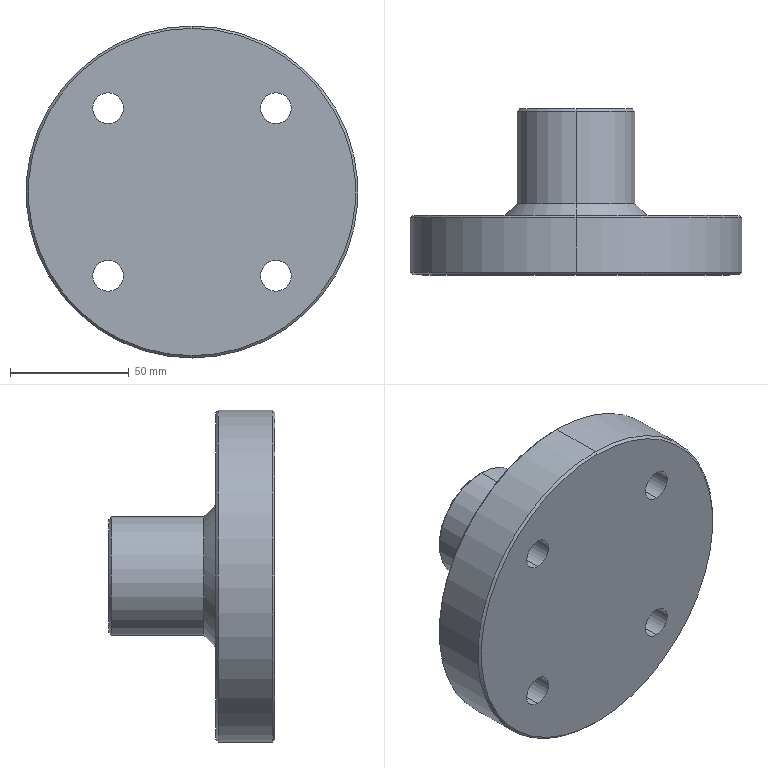Part | SolidWorks | features BaseBody 1 | 1 solid | 30 faces | box 140 x 70 x 140 mm | volume 427164 mm3 | cylinder 14 | cone 12 | plane 4 | commonest cylinder face diameters 13 x8 30 x2 50 x2 140 x2
STEP:
#1=CARTESIAN_POINT('',(35.355,0.,28.855));
#2=VERTEX_POINT('',#1);
#3=CARTESIAN_POINT('',(35.355,0.,41.855));
#4=VERTEX_POINT('',#3);
#5=CARTESIAN_POINT('',(35.355,0.,35.355));
#6=DIRECTION('',(0.,1.,0.));
#7=DIRECTION('',(0.,0.,1.));
#8=AXIS2_PLACEMENT_3D('',#5,#6,#7);
#9=CIRCLE('',#8,6.5);
#10=EDGE_CURVE('',#2,#4,#9,.T.);
#11=ORIENTED_EDGE('',*,*,#10,.F.);
#12=CARTESIAN_POINT('',(35.355,25.,28.855));
#13=VERTEX_POINT('',#12);
#14=CARTESIAN_POINT('',(35.355,25.,28.855));
#15=DIRECTION('',(0.,1.,0.));
#16=VECTOR('',#15,1000.);
#17=LINE('',#14,#16);
#18=EDGE_CURVE('',#2,#13,#17,.T.);
#19=ORIENTED_EDGE('',*,*,#18,.T.);
#20=CARTESIAN_POINT('',(35.355,25.,41.855));
#21=VERTEX_POINT('',#20);
#22=CARTESIAN_POINT('',(35.355,25.,35.355));
#23=DIRECTION('',(0.,1.,0.));
#24=DIRECTION('',(0.,0.,1.));
#25=AXIS2_PLACEMENT_3D('',#22,#23,#24);
#26=CIRCLE('',#25,6.5);
#27=EDGE_CURVE('',#13,#21,#26,.T.);
#28=ORIENTED_EDGE('',*,*,#27,.T.);
#29=CARTESIAN_POINT('',(35.355,25.,41.855));
#30=DIRECTION('',(0.,1.,0.));
#31=VECTOR('',#30,1000.);
#32=LINE('',#29,#31);
#33=EDGE_CURVE('',#4,#21,#32,.T.);
#34=ORIENTED_EDGE('',*,*,#33,.F.);
#35=EDGE_LOOP('',(#11,#19,#28,#34));
#36=FACE_OUTER_BOUND('',#35,.T.);
#37=CARTESIAN_POINT('',(35.355,25.,35.355));
#38=DIRECTION('',(0.,1.,0.));
#39=DIRECTION('',(0.,0.,1.));
#40=AXIS2_PLACEMENT_3D('',#37,#38,#39);
#41=CYLINDRICAL_SURFACE('',#40,6.5);
#42=ADVANCED_FACE('',(#36),#41,.F.);
#43=CARTESIAN_POINT('',(-35.355,0.,28.855));
#44=VERTEX_POINT('',#43);
#45=CARTESIAN_POINT('',(-35.355,0.,41.855));
#46=VERTEX_POINT('',#45);
#47=CARTESIAN_POINT('',(-35.355,0.,35.355));
#48=DIRECTION('',(0.,1.,0.));
#49=DIRECTION('',(0.,0.,1.));
#50=AXIS2_PLACEMENT_3D('',#47,#48,#49);
#51=CIRCLE('',#50,6.5);
#52=EDGE_CURVE('',#44,#46,#51,.T.);
#53=ORIENTED_EDGE('',*,*,#52,.F.);
#54=CARTESIAN_POINT('',(-35.355,25.,28.855));
#55=VERTEX_POINT('',#54);
#56=CARTESIAN_POINT('',(-35.355,25.,28.855));
#57=DIRECTION('',(0.,1.,0.));
#58=VECTOR('',#57,1000.);
#59=LINE('',#56,#58);
#60=EDGE_CURVE('',#44,#55,#59,.T.);
#61=ORIENTED_EDGE('',*,*,#60,.T.);
#62=CARTESIAN_POINT('',(-35.355,25.,41.855));
#63=VERTEX_POINT('',#62);
#64=CARTESIAN_POINT('',(-35.355,25.,35.355));
#65=DIRECTION('',(0.,1.,0.));
#66=DIRECTION('',(0.,0.,1.));
#67=AXIS2_PLACEMENT_3D('',#64,#65,#66);
#68=CIRCLE('',#67,6.5);
#69=EDGE_CURVE('',#55,#63,#68,.T.);
#70=ORIENTED_EDGE('',*,*,#69,.T.);
#71=CARTESIAN_POINT('',(-35.355,25.,41.855));
#72=DIRECTION('',(0.,1.,0.));
#73=VECTOR('',#72,1000.);
#74=LINE('',#71,#73);
#75=EDGE_CURVE('',#46,#63,#74,.T.);
#76=ORIENTED_EDGE('',*,*,#75,.F.);
#77=EDGE_LOOP('',(#53,#61,#70,#76));
#78=FACE_OUTER_BOUND('',#77,.T.);
#79=CARTESIAN_POINT('',(-35.355,25.,35.355));
#80=DIRECTION('',(0.,1.,0.));
#81=DIRECTION('',(0.,0.,1.));
#82=AXIS2_PLACEMENT_3D('',#79,#80,#81);
#83=CYLINDRICAL_SURFACE('',#82,6.5);
#84=ADVANCED_FACE('',(#78),#83,.F.);
#85=CARTESIAN_POINT('',(-35.355,0.,-41.855));
#86=VERTEX_POINT('',#85);
#87=CARTESIAN_POINT('',(-35.355,0.,-28.855));
#88=VERTEX_POINT('',#87);
#89=CARTESIAN_POINT('',(-35.355,0.,-35.355));
#90=DIRECTION('',(0.,1.,0.));
#91=DIRECTION('',(0.,0.,1.));
#92=AXIS2_PLACEMENT_3D('',#89,#90,#91);
#93=CIRCLE('',#92,6.5);
#94=EDGE_CURVE('',#86,#88,#93,.T.);
#95=ORIENTED_EDGE('',*,*,#94,.F.);
#96=CARTESIAN_POINT('',(-35.355,25.,-41.855));
#97=VERTEX_POINT('',#96);
#98=CARTESIAN_POINT('',(-35.355,25.,-41.855));
#99=DIRECTION('',(0.,1.,0.));
#100=VECTOR('',#99,1000.);
#101=LINE('',#98,#100);
#102=EDGE_CURVE('',#86,#97,#101,.T.);
#103=ORIENTED_EDGE('',*,*,#102,.T.);
#104=CARTESIAN_POINT('',(-35.355,25.,-28.855));
#105=VERTEX_POINT('',#104);
#106=CARTESIAN_POINT('',(-35.355,25.,-35.355));
#107=DIRECTION('',(0.,1.,0.));
#108=DIRECTION('',(0.,0.,1.));
#109=AXIS2_PLACEMENT_3D('',#106,#107,#108);
#110=CIRCLE('',#109,6.5);
#111=EDGE_CURVE('',#97,#105,#110,.T.);
#112=ORIENTED_EDGE('',*,*,#111,.T.);
#113=CARTESIAN_POINT('',(-35.355,25.,-28.855));
#114=DIRECTION('',(0.,1.,0.));
#115=VECTOR('',#114,1000.);
#116=LINE('',#113,#115);
#117=EDGE_CURVE('',#88,#105,#116,.T.);
#118=ORIENTED_EDGE('',*,*,#117,.F.);
#119=EDGE_LOOP('',(#95,#103,#112,#118));
#120=FACE_OUTER_BOUND('',#119,.T.);
#121=CARTESIAN_POINT('',(-35.355,25.,-35.355));
#122=DIRECTION('',(0.,1.,0.));
#123=DIRECTION('',(0.,0.,1.));
#124=AXIS2_PLACEMENT_3D('',#121,#122,#123);
#125=CYLINDRICAL_SURFACE('',#124,6.5);
#126=ADVANCED_FACE('',(#120),#125,.F.);
#127=CARTESIAN_POINT('',(35.355,0.,-41.855));
#128=VERTEX_POINT('',#127);
#129=CARTESIAN_POINT('',(35.355,0.,-28.855));
#130=VERTEX_POINT('',#129);
#131=CARTESIAN_POINT('',(35.355,0.,-35.355));
#132=DIRECTION('',(0.,1.,0.));
#133=DIRECTION('',(0.,0.,1.));
#134=AXIS2_PLACEMENT_3D('',#131,#132,#133);
#135=CIRCLE('',#134,6.5);
#136=EDGE_CURVE('',#128,#130,#135,.T.);
#137=ORIENTED_EDGE('',*,*,#136,.F.);
#138=CARTESIAN_POINT('',(35.355,25.,-41.855));
#139=VERTEX_POINT('',#138);
#140=CARTESIAN_POINT('',(35.355,25.,-41.855));
#141=DIRECTION('',(0.,1.,0.));
#142=VECTOR('',#141,1000.);
#143=LINE('',#140,#142);
#144=EDGE_CURVE('',#128,#139,#143,.T.);
#145=ORIENTED_EDGE('',*,*,#144,.T.);
#146=CARTESIAN_POINT('',(35.355,25.,-28.855));
#147=VERTEX_POINT('',#146);
#148=CARTESIAN_POINT('',(35.355,25.,-35.355));
#149=DIRECTION('',(0.,1.,0.));
#150=DIRECTION('',(0.,0.,1.));
#151=AXIS2_PLACEMENT_3D('',#148,#149,#150);
#152=CIRCLE('',#151,6.5);
#153=EDGE_CURVE('',#139,#147,#152,.T.);
#154=ORIENTED_EDGE('',*,*,#153,.T.);
#155=CARTESIAN_POINT('',(35.355,25.,-28.855));
#156=DIRECTION('',(0.,1.,0.));
#157=VECTOR('',#156,1000.);
#158=LINE('',#155,#157);
#159=EDGE_CURVE('',#130,#147,#158,.T.);
#160=ORIENTED_EDGE('',*,*,#159,.F.);
#161=EDGE_LOOP('',(#137,#145,#154,#160));
#162=FACE_OUTER_BOUND('',#161,.T.);
#163=CARTESIAN_POINT('',(35.355,25.,-35.355));
#164=DIRECTION('',(0.,1.,0.));
#165=DIRECTION('',(0.,0.,1.));
#166=AXIS2_PLACEMENT_3D('',#163,#164,#165);
#167=CYLINDRICAL_SURFACE('',#166,6.5);
#168=ADVANCED_FACE('',(#162),#167,.F.);
#169=CARTESIAN_POINT('',(0.,20.,-10.));
#170=VERTEX_POINT('',#169);
#171=CARTESIAN_POINT('',(0.,20.,10.));
#172=VERTEX_POINT('',#171);
#173=CARTESIAN_POINT('',(0.,20.,0.));
#174=DIRECTION('',(0.,1.,0.));
#175=DIRECTION('',(0.,0.,1.));
#176=AXIS2_PLACEMENT_3D('',#173,#174,#175);
#177=CIRCLE('',#176,10.);
#178=EDGE_CURVE('',#170,#172,#177,.T.);
#179=ORIENTED_EDGE('',*,*,#178,.F.);
#180=CARTESIAN_POINT('',(0.,25.,-15.));
#181=VERTEX_POINT('',#180);
#182=CARTESIAN_POINT('',(0.,25.,-15.));
#183=DIRECTION('',(0.,0.7071,-0.7071));
#184=VECTOR('',#183,1000.);
#185=LINE('',#182,#184);
#186=EDGE_CURVE('',#170,#181,#185,.T.);
#187=ORIENTED_EDGE('',*,*,#186,.T.);
#188=CARTESIAN_POINT('',(0.,25.,15.));
#189=VERTEX_POINT('',#188);
#190=CARTESIAN_POINT('',(0.,25.,0.));
#191=DIRECTION('',(0.,1.,0.));
#192=DIRECTION('',(0.,0.,1.));
#193=AXIS2_PLACEMENT_3D('',#190,#191,#192);
#194=CIRCLE('',#193,15.);
#195=EDGE_CURVE('',#181,#189,#194,.T.);
#196=ORIENTED_EDGE('',*,*,#195,.T.);
#197=CARTESIAN_POINT('',(0.,25.,15.));
#198=DIRECTION('',(0.,0.7071,0.7071));
#199=VECTOR('',#198,1000.);
#200=LINE('',#197,#199);
#201=EDGE_CURVE('',#172,#189,#200,.T.);
#202=ORIENTED_EDGE('',*,*,#201,.F.);
#203=EDGE_LOOP('',(#179,#187,#196,#202));
#204=FACE_OUTER_BOUND('',#203,.T.);
#205=CARTESIAN_POINT('',(0.,25.,0.));
#206=DIRECTION('',(0.,1.,0.));
#207=DIRECTION('',(0.,0.,1.));
#208=AXIS2_PLACEMENT_3D('',#205,#206,#207);
#209=CONICAL_SURFACE('',#208,15.,0.7854);
#210=ADVANCED_FACE('',(#204),#209,.F.);
#211=ORIENTED_EDGE('',*,*,#195,.F.);
#212=CARTESIAN_POINT('',(0.,69.,-15.));
#213=VERTEX_POINT('',#212);
#214=CARTESIAN_POINT('',(0.,20.,-15.));
#215=DIRECTION('',(0.,1.,0.));
#216=VECTOR('',#215,1000.);
#217=LINE('',#214,#216);
#218=EDGE_CURVE('',#181,#213,#217,.T.);
#219=ORIENTED_EDGE('',*,*,#218,.T.);
#220=CARTESIAN_POINT('',(0.,69.,15.));
#221=VERTEX_POINT('',#220);
#222=CARTESIAN_POINT('',(0.,69.,0.));
#223=DIRECTION('',(0.,1.,0.));
#224=DIRECTION('',(0.,0.,1.));
#225=AXIS2_PLACEMENT_3D('',#222,#223,#224);
#226=CIRCLE('',#225,15.);
#227=EDGE_CURVE('',#213,#221,#226,.T.);
#228=ORIENTED_EDGE('',*,*,#227,.T.);
#229=CARTESIAN_POINT('',(0.,20.,15.));
#230=DIRECTION('',(0.,1.,0.));
#231=VECTOR('',#230,1000.);
#232=LINE('',#229,#231);
#233=EDGE_CURVE('',#189,#221,#232,.T.);
#234=ORIENTED_EDGE('',*,*,#233,.F.);
#235=EDGE_LOOP('',(#211,#219,#228,#234));
#236=FACE_OUTER_BOUND('',#235,.T.);
#237=CARTESIAN_POINT('',(0.,20.,0.));
#238=DIRECTION('',(0.,1.,0.));
#239=DIRECTION('',(0.,0.,1.));
#240=AXIS2_PLACEMENT_3D('',#237,#238,#239);
#241=CYLINDRICAL_SURFACE('',#240,15.);
#242=ADVANCED_FACE('',(#236),#241,.F.);
#243=ORIENTED_EDGE('',*,*,#227,.F.);
#244=CARTESIAN_POINT('',(0.,70.,-16.));
#245=VERTEX_POINT('',#244);
#246=CARTESIAN_POINT('',(0.,70.,-16.));
#247=DIRECTION('',(0.,0.7071,-0.7071));
#248=VECTOR('',#247,1000.);
#249=LINE('',#246,#248);
#250=EDGE_CURVE('',#213,#245,#249,.T.);
#251=ORIENTED_EDGE('',*,*,#250,.T.);
#252=CARTESIAN_POINT('',(0.,70.,16.));
#253=VERTEX_POINT('',#252);
#254=CARTESIAN_POINT('',(0.,70.,0.));
#255=DIRECTION('',(0.,1.,0.));
#256=DIRECTION('',(0.,0.,1.));
#257=AXIS2_PLACEMENT_3D('',#254,#255,#256);
#258=CIRCLE('',#257,16.);
#259=EDGE_CURVE('',#245,#253,#258,.T.);
#260=ORIENTED_EDGE('',*,*,#259,.T.);
#261=CARTESIAN_POINT('',(0.,70.,16.));
#262=DIRECTION('',(0.,0.7071,0.7071));
#263=VECTOR('',#262,1000.);
#264=LINE('',#261,#263);
#265=EDGE_CURVE('',#221,#253,#264,.T.);
#266=ORIENTED_EDGE('',*,*,#265,.F.);
#267=EDGE_LOOP('',(#243,#251,#260,#266));
#268=FACE_OUTER_BOUND('',#267,.T.);
#269=CARTESIAN_POINT('',(0.,70.,0.));
#270=DIRECTION('',(0.,1.,0.));
#271=DIRECTION('',(0.,0.,1.));
#272=AXIS2_PLACEMENT_3D('',#269,#270,#271);
#273=CONICAL_SURFACE('',#272,16.,0.7854);
#274=ADVANCED_FACE('',(#268),#273,.F.);
#275=CARTESIAN_POINT('',(0.,70.,24.));
#276=VERTEX_POINT('',#275);
#277=CARTESIAN_POINT('',(0.,70.,-24.));
#278=VERTEX_POINT('',#277);
#279=CARTESIAN_POINT('',(0.,70.,0.));
#280=DIRECTION('',(0.,1.,0.));
#281=DIRECTION('',(0.,0.,1.));
#282=AXIS2_PLACEMENT_3D('',#279,#280,#281);
#283=CIRCLE('',#282,24.);
#284=EDGE_CURVE('',#276,#278,#283,.T.);
#285=ORIENTED_EDGE('',*,*,#284,.F.);
#286=CARTESIAN_POINT('',(0.,69.,25.));
#287=VERTEX_POINT('',#286);
#288=CARTESIAN_POINT('',(0.,69.,25.));
#289=DIRECTION('',(0.,-0.7071,0.7071));
#290=VECTOR('',#289,1000.);
#291=LINE('',#288,#290);
#292=EDGE_CURVE('',#276,#287,#291,.T.);
#293=ORIENTED_EDGE('',*,*,#292,.T.);
#294=CARTESIAN_POINT('',(0.,69.,-25.));
#295=VERTEX_POINT('',#294);
#296=CARTESIAN_POINT('',(0.,69.,0.));
#297=DIRECTION('',(0.,1.,0.));
#298=DIRECTION('',(0.,0.,1.));
#299=AXIS2_PLACEMENT_3D('',#296,#297,#298);
#300=CIRCLE('',#299,25.);
#301=EDGE_CURVE('',#287,#295,#300,.T.);
#302=ORIENTED_EDGE('',*,*,#301,.T.);
#303=CARTESIAN_POINT('',(0.,69.,-25.));
#304=DIRECTION('',(0.,-0.7071,-0.7071));
#305=VECTOR('',#304,1000.);
#306=LINE('',#303,#305);
#307=EDGE_CURVE('',#278,#295,#306,.T.);
#308=ORIENTED_EDGE('',*,*,#307,.F.);
#309=EDGE_LOOP('',(#285,#293,#302,#308));
#310=FACE_OUTER_BOUND('',#309,.T.);
#311=CARTESIAN_POINT('',(0.,69.,0.));
#312=DIRECTION('',(0.,-1.,0.));
#313=DIRECTION('',(0.,0.,-1.));
#314=AXIS2_PLACEMENT_3D('',#311,#312,#313);
#315=CONICAL_SURFACE('',#314,25.,0.7854);
#316=ADVANCED_FACE('',(#310),#315,.T.);
#317=CARTESIAN_POINT('',(0.,30.,25.));
#318=VERTEX_POINT('',#317);
#319=CARTESIAN_POINT('',(0.,30.,-25.));
#320=VERTEX_POINT('',#319);
#321=CARTESIAN_POINT('',(0.,30.,0.));
#322=DIRECTION('',(0.,1.,0.));
#323=DIRECTION('',(0.,0.,1.));
#324=AXIS2_PLACEMENT_3D('',#321,#322,#323);
#325=CIRCLE('',#324,25.);
#326=EDGE_CURVE('',#318,#320,#325,.T.);
#327=ORIENTED_EDGE('',*,*,#326,.T.);
#328=CARTESIAN_POINT('',(0.,20.,-25.));
#329=DIRECTION('',(0.,1.,0.));
#330=VECTOR('',#329,1000.);
#331=LINE('',#328,#330);
#332=EDGE_CURVE('',#320,#295,#331,.T.);
#333=ORIENTED_EDGE('',*,*,#332,.T.);
#334=ORIENTED_EDGE('',*,*,#301,.F.);
#335=CARTESIAN_POINT('',(0.,20.,25.));
#336=DIRECTION('',(0.,1.,0.));
#337=VECTOR('',#336,1000.);
#338=LINE('',#335,#337);
#339=EDGE_CURVE('',#318,#287,#338,.T.);
#340=ORIENTED_EDGE('',*,*,#339,.F.);
#341=EDGE_LOOP('',(#327,#333,#334,#340));
#342=FACE_OUTER_BOUND('',#341,.T.);
#343=CARTESIAN_POINT('',(0.,20.,0.));
#344=DIRECTION('',(0.,1.,0.));
#345=DIRECTION('',(0.,0.,1.));
#346=AXIS2_PLACEMENT_3D('',#343,#344,#345);
#347=CYLINDRICAL_SURFACE('',#346,25.);
#348=ADVANCED_FACE('',(#342),#347,.T.);
#349=ORIENTED_EDGE('',*,*,#326,.F.);
#350=CARTESIAN_POINT('',(0.,25.,30.));
#351=VERTEX_POINT('',#350);
#352=CARTESIAN_POINT('',(0.,25.,30.));
#353=DIRECTION('',(0.,-0.7071,0.7071));
#354=VECTOR('',#353,1000.);
#355=LINE('',#352,#354);
#356=EDGE_CURVE('',#318,#351,#355,.T.);
#357=ORIENTED_EDGE('',*,*,#356,.T.);
#358=CARTESIAN_POINT('',(0.,25.,-30.));
#359=VERTEX_POINT('',#358);
#360=CARTESIAN_POINT('',(0.,25.,0.));
#361=DIRECTION('',(0.,1.,0.));
#362=DIRECTION('',(0.,0.,1.));
#363=AXIS2_PLACEMENT_3D('',#360,#361,#362);
#364=CIRCLE('',#363,30.);
#365=EDGE_CURVE('',#351,#359,#364,.T.);
#366=ORIENTED_EDGE('',*,*,#365,.T.);
#367=CARTESIAN_POINT('',(0.,25.,-30.));
#368=DIRECTION('',(0.,-0.7071,-0.7071));
#369=VECTOR('',#368,1000.);
#370=LINE('',#367,#369);
#371=EDGE_CURVE('',#320,#359,#370,.T.);
#372=ORIENTED_EDGE('',*,*,#371,.F.);
#373=EDGE_LOOP('',(#349,#357,#366,#372));
#374=FACE_OUTER_BOUND('',#373,.T.);
#375=CARTESIAN_POINT('',(0.,25.,0.));
#376=DIRECTION('',(0.,-1.,0.));
#377=DIRECTION('',(0.,0.,-1.));
#378=AXIS2_PLACEMENT_3D('',#375,#376,#377);
#379=CONICAL_SURFACE('',#378,30.,0.7854);
#380=ADVANCED_FACE('',(#374),#379,.T.);
#381=CARTESIAN_POINT('',(0.,25.,69.));
#382=VERTEX_POINT('',#381);
#383=CARTESIAN_POINT('',(0.,25.,-69.));
#384=VERTEX_POINT('',#383);
#385=CARTESIAN_POINT('',(0.,25.,0.));
#386=DIRECTION('',(0.,1.,0.));
#387=DIRECTION('',(0.,0.,1.));
#388=AXIS2_PLACEMENT_3D('',#385,#386,#387);
#389=CIRCLE('',#388,69.);
#390=EDGE_CURVE('',#382,#384,#389,.T.);
#391=ORIENTED_EDGE('',*,*,#390,.F.);
#392=CARTESIAN_POINT('',(0.,24.,70.));
#393=VERTEX_POINT('',#392);
#394=CARTESIAN_POINT('',(0.,24.,70.));
#395=DIRECTION('',(0.,-0.7071,0.7071));
#396=VECTOR('',#395,1000.);
#397=LINE('',#394,#396);
#398=EDGE_CURVE('',#382,#393,#397,.T.);
#399=ORIENTED_EDGE('',*,*,#398,.T.);
#400=CARTESIAN_POINT('',(0.,24.,-70.));
#401=VERTEX_POINT('',#400);
#402=CARTESIAN_POINT('',(0.,24.,0.));
#403=DIRECTION('',(0.,1.,0.));
#404=DIRECTION('',(0.,0.,1.));
#405=AXIS2_PLACEMENT_3D('',#402,#403,#404);
#406=CIRCLE('',#405,70.);
#407=EDGE_CURVE('',#393,#401,#406,.T.);
#408=ORIENTED_EDGE('',*,*,#407,.T.);
#409=CARTESIAN_POINT('',(0.,24.,-70.));
#410=DIRECTION('',(0.,-0.7071,-0.7071));
#411=VECTOR('',#410,1000.);
#412=LINE('',#409,#411);
#413=EDGE_CURVE('',#384,#401,#412,.T.);
#414=ORIENTED_EDGE('',*,*,#413,.F.);
#415=EDGE_LOOP('',(#391,#399,#408,#414));
#416=FACE_OUTER_BOUND('',#415,.T.);
#417=CARTESIAN_POINT('',(0.,24.,0.));
#418=DIRECTION('',(0.,-1.,0.));
#419=DIRECTION('',(0.,0.,-1.));
#420=AXIS2_PLACEMENT_3D('',#417,#418,#419);
#421=CONICAL_SURFACE('',#420,70.,0.7854);
#422=ADVANCED_FACE('',(#416),#421,.T.);
#423=CARTESIAN_POINT('',(0.,1.,70.));
#424=VERTEX_POINT('',#423);
#425=CARTESIAN_POINT('',(0.,1.,-70.));
#426=VERTEX_POINT('',#425);
#427=CARTESIAN_POINT('',(0.,1.,0.));
#428=DIRECTION('',(0.,1.,0.));
#429=DIRECTION('',(0.,0.,1.));
#430=AXIS2_PLACEMENT_3D('',#427,#428,#429);
#431=CIRCLE('',#430,70.);
#432=EDGE_CURVE('',#424,#426,#431,.T.);
#433=ORIENTED_EDGE('',*,*,#432,.T.);
#434=CARTESIAN_POINT('',(0.,20.,-70.));
#435=DIRECTION('',(0.,1.,0.));
#436=VECTOR('',#435,1000.);
#437=LINE('',#434,#436);
#438=EDGE_CURVE('',#426,#401,#437,.T.);
#439=ORIENTED_EDGE('',*,*,#438,.T.);
#440=ORIENTED_EDGE('',*,*,#407,.F.);
#441=CARTESIAN_POINT('',(0.,20.,70.));
#442=DIRECTION('',(0.,1.,0.));
#443=VECTOR('',#442,1000.);
#444=LINE('',#441,#443);
#445=EDGE_CURVE('',#424,#393,#444,.T.);
#446=ORIENTED_EDGE('',*,*,#445,.F.);
#447=EDGE_LOOP('',(#433,#439,#440,#446));
#448=FACE_OUTER_BOUND('',#447,.T.);
#449=CARTESIAN_POINT('',(0.,20.,0.));
#450=DIRECTION('',(0.,1.,0.));
#451=DIRECTION('',(0.,0.,1.));
#452=AXIS2_PLACEMENT_3D('',#449,#450,#451);
#453=CYLINDRICAL_SURFACE('',#452,70.);
#454=ADVANCED_FACE('',(#448),#453,.T.);
#455=CARTESIAN_POINT('',(0.,0.,69.));
#456=VERTEX_POINT('',#455);
#457=CARTESIAN_POINT('',(0.,0.,-69.));
#458=VERTEX_POINT('',#457);
#459=CARTESIAN_POINT('',(0.,0.,0.));
#460=DIRECTION('',(0.,1.,0.));
#461=DIRECTION('',(0.,0.,1.));
#462=AXIS2_PLACEMENT_3D('',#459,#460,#461);
#463=CIRCLE('',#462,69.);
#464=EDGE_CURVE('',#456,#458,#463,.T.);
#465=ORIENTED_EDGE('',*,*,#464,.T.);
#466=CARTESIAN_POINT('',(0.,0.,-69.));
#467=DIRECTION('',(0.,0.7071,-0.7071));
#468=VECTOR('',#467,1000.);
#469=LINE('',#466,#468);
#470=EDGE_CURVE('',#458,#426,#469,.T.);
#471=ORIENTED_EDGE('',*,*,#470,.T.);
#472=ORIENTED_EDGE('',*,*,#432,.F.);
#473=CARTESIAN_POINT('',(0.,0.,69.));
#474=DIRECTION('',(0.,0.7071,0.7071));
#475=VECTOR('',#474,1000.);
#476=LINE('',#473,#475);
#477=EDGE_CURVE('',#456,#424,#476,.T.);
#478=ORIENTED_EDGE('',*,*,#477,.F.);
#479=EDGE_LOOP('',(#465,#471,#472,#478));
#480=FACE_OUTER_BOUND('',#479,.T.);
#481=CARTESIAN_POINT('',(0.,0.,0.));
#482=DIRECTION('',(0.,1.,0.));
#483=DIRECTION('',(0.,0.,1.));
#484=AXIS2_PLACEMENT_3D('',#481,#482,#483);
#485=CONICAL_SURFACE('',#484,69.,0.7854);
#486=ADVANCED_FACE('',(#480),#485,.T.);
#487=CARTESIAN_POINT('',(35.355,0.,35.355));
#488=DIRECTION('',(0.,1.,0.));
#489=DIRECTION('',(0.,0.,1.));
#490=AXIS2_PLACEMENT_3D('',#487,#488,#489);
#491=CIRCLE('',#490,6.5);
#492=EDGE_CURVE('',#4,#2,#491,.T.);
#493=ORIENTED_EDGE('',*,*,#492,.T.);
#494=ORIENTED_EDGE('',*,*,#10,.T.);
#495=EDGE_LOOP('',(#493,#494));
#496=FACE_BOUND('',#495,.T.);
#497=CARTESIAN_POINT('',(-35.355,0.,35.355));
#498=DIRECTION('',(0.,1.,0.));
#499=DIRECTION('',(0.,0.,1.));
#500=AXIS2_PLACEMENT_3D('',#497,#498,#499);
#501=CIRCLE('',#500,6.5);
#502=EDGE_CURVE('',#46,#44,#501,.T.);
#503=ORIENTED_EDGE('',*,*,#502,.T.);
#504=ORIENTED_EDGE('',*,*,#52,.T.);
#505=EDGE_LOOP('',(#503,#504));
#506=FACE_BOUND('',#505,.T.);
#507=CARTESIAN_POINT('',(-35.355,0.,-35.355));
#508=DIRECTION('',(0.,1.,0.));
#509=DIRECTION('',(0.,0.,1.));
#510=AXIS2_PLACEMENT_3D('',#507,#508,#509);
#511=CIRCLE('',#510,6.5);
#512=EDGE_CURVE('',#88,#86,#511,.T.);
#513=ORIENTED_EDGE('',*,*,#512,.T.);
#514=ORIENTED_EDGE('',*,*,#94,.T.);
#515=EDGE_LOOP('',(#513,#514));
#516=FACE_BOUND('',#515,.T.);
#517=CARTESIAN_POINT('',(35.355,0.,-35.355));
#518=DIRECTION('',(0.,1.,0.));
#519=DIRECTION('',(0.,0.,1.));
#520=AXIS2_PLACEMENT_3D('',#517,#518,#519);
#521=CIRCLE('',#520,6.5);
#522=EDGE_CURVE('',#130,#128,#521,.T.);
#523=ORIENTED_EDGE('',*,*,#522,.T.);
#524=ORIENTED_EDGE('',*,*,#136,.T.);
#525=EDGE_LOOP('',(#523,#524));
#526=FACE_BOUND('',#525,.T.);
#527=ORIENTED_EDGE('',*,*,#464,.F.);
#528=CARTESIAN_POINT('',(0.,0.,0.));
#529=DIRECTION('',(0.,1.,0.));
#530=DIRECTION('',(0.,0.,1.));
#531=AXIS2_PLACEMENT_3D('',#528,#529,#530);
#532=CIRCLE('',#531,69.);
#533=EDGE_CURVE('',#458,#456,#532,.T.);
#534=ORIENTED_EDGE('',*,*,#533,.F.);
#535=EDGE_LOOP('',(#527,#534));
#536=FACE_OUTER_BOUND('',#535,.T.);
#537=CARTESIAN_POINT('',(0.,0.,0.));
#538=DIRECTION('',(0.,1.,0.));
#539=DIRECTION('',(0.,0.,1.));
#540=AXIS2_PLACEMENT_3D('',#537,#538,#539);
#541=PLANE('',#540);
#542=ADVANCED_FACE('',(#496,#506,#516,#526,#536),#541,.F.);
#543=ORIENTED_EDGE('',*,*,#470,.F.);
#544=ORIENTED_EDGE('',*,*,#533,.T.);
#545=ORIENTED_EDGE('',*,*,#477,.T.);
#546=CARTESIAN_POINT('',(0.,1.,0.));
#547=DIRECTION('',(0.,1.,0.));
#548=DIRECTION('',(0.,0.,1.));
#549=AXIS2_PLACEMENT_3D('',#546,#547,#548);
#550=CIRCLE('',#549,70.);
#551=EDGE_CURVE('',#426,#424,#550,.T.);
#552=ORIENTED_EDGE('',*,*,#551,.F.);
#553=EDGE_LOOP('',(#543,#544,#545,#552));
#554=FACE_OUTER_BOUND('',#553,.T.);
#555=CARTESIAN_POINT('',(0.,0.,0.));
#556=DIRECTION('',(0.,1.,0.));
#557=DIRECTION('',(0.,0.,1.));
#558=AXIS2_PLACEMENT_3D('',#555,#556,#557);
#559=CONICAL_SURFACE('',#558,69.,0.7854);
#560=ADVANCED_FACE('',(#554),#559,.T.);
#561=ORIENTED_EDGE('',*,*,#438,.F.);
#562=ORIENTED_EDGE('',*,*,#551,.T.);
#563=ORIENTED_EDGE('',*,*,#445,.T.);
#564=CARTESIAN_POINT('',(0.,24.,0.));
#565=DIRECTION('',(0.,1.,0.));
#566=DIRECTION('',(0.,0.,1.));
#567=AXIS2_PLACEMENT_3D('',#564,#565,#566);
#568=CIRCLE('',#567,70.);
#569=EDGE_CURVE('',#401,#393,#568,.T.);
#570=ORIENTED_EDGE('',*,*,#569,.F.);
#571=EDGE_LOOP('',(#561,#562,#563,#570));
#572=FACE_OUTER_BOUND('',#571,.T.);
#573=CARTESIAN_POINT('',(0.,20.,0.));
#574=DIRECTION('',(0.,1.,0.));
#575=DIRECTION('',(0.,0.,1.));
#576=AXIS2_PLACEMENT_3D('',#573,#574,#575);
#577=CYLINDRICAL_SURFACE('',#576,70.);
#578=ADVANCED_FACE('',(#572),#577,.T.);
#579=ORIENTED_EDGE('',*,*,#398,.F.);
#580=CARTESIAN_POINT('',(0.,25.,0.));
#581=DIRECTION('',(0.,1.,0.));
#582=DIRECTION('',(0.,0.,1.));
#583=AXIS2_PLACEMENT_3D('',#580,#581,#582);
#584=CIRCLE('',#583,69.);
#585=EDGE_CURVE('',#384,#382,#584,.T.);
#586=ORIENTED_EDGE('',*,*,#585,.F.);
#587=ORIENTED_EDGE('',*,*,#413,.T.);
#588=ORIENTED_EDGE('',*,*,#569,.T.);
#589=EDGE_LOOP('',(#579,#586,#587,#588));
#590=FACE_OUTER_BOUND('',#589,.T.);
#591=CARTESIAN_POINT('',(0.,24.,0.));
#592=DIRECTION('',(0.,-1.,0.));
#593=DIRECTION('',(0.,0.,-1.));
#594=AXIS2_PLACEMENT_3D('',#591,#592,#593);
#595=CONICAL_SURFACE('',#594,70.,0.7854);
#596=ADVANCED_FACE('',(#590),#595,.T.);
#597=CARTESIAN_POINT('',(35.355,25.,35.355));
#598=DIRECTION('',(0.,1.,0.));
#599=DIRECTION('',(0.,0.,1.));
#600=AXIS2_PLACEMENT_3D('',#597,#598,#599);
#601=CIRCLE('',#600,6.5);
#602=EDGE_CURVE('',#21,#13,#601,.T.);
#603=ORIENTED_EDGE('',*,*,#602,.F.);
#604=ORIENTED_EDGE('',*,*,#27,.F.);
#605=EDGE_LOOP('',(#603,#604));
#606=FACE_BOUND('',#605,.T.);
#607=CARTESIAN_POINT('',(-35.355,25.,35.355));
#608=DIRECTION('',(0.,1.,0.));
#609=DIRECTION('',(0.,0.,1.));
#610=AXIS2_PLACEMENT_3D('',#607,#608,#609);
#611=CIRCLE('',#610,6.5);
#612=EDGE_CURVE('',#63,#55,#611,.T.);
#613=ORIENTED_EDGE('',*,*,#612,.F.);
#614=ORIENTED_EDGE('',*,*,#69,.F.);
#615=EDGE_LOOP('',(#613,#614));
#616=FACE_BOUND('',#615,.T.);
#617=CARTESIAN_POINT('',(-35.355,25.,-35.355));
#618=DIRECTION('',(0.,1.,0.));
#619=DIRECTION('',(0.,0.,1.));
#620=AXIS2_PLACEMENT_3D('',#617,#618,#619);
#621=CIRCLE('',#620,6.5);
#622=EDGE_CURVE('',#105,#97,#621,.T.);
#623=ORIENTED_EDGE('',*,*,#622,.F.);
#624=ORIENTED_EDGE('',*,*,#111,.F.);
#625=EDGE_LOOP('',(#623,#624));
#626=FACE_BOUND('',#625,.T.);
#627=CARTESIAN_POINT('',(35.355,25.,-35.355));
#628=DIRECTION('',(0.,1.,0.));
#629=DIRECTION('',(0.,0.,1.));
#630=AXIS2_PLACEMENT_3D('',#627,#628,#629);
#631=CIRCLE('',#630,6.5);
#632=EDGE_CURVE('',#147,#139,#631,.T.);
#633=ORIENTED_EDGE('',*,*,#632,.F.);
#634=ORIENTED_EDGE('',*,*,#153,.F.);
#635=EDGE_LOOP('',(#633,#634));
#636=FACE_BOUND('',#635,.T.);
#637=CARTESIAN_POINT('',(0.,25.,0.));
#638=DIRECTION('',(0.,1.,0.));
#639=DIRECTION('',(0.,0.,1.));
#640=AXIS2_PLACEMENT_3D('',#637,#638,#639);
#641=CIRCLE('',#640,30.);
#642=EDGE_CURVE('',#359,#351,#641,.T.);
#643=ORIENTED_EDGE('',*,*,#642,.F.);
#644=ORIENTED_EDGE('',*,*,#365,.F.);
#645=EDGE_LOOP('',(#643,#644));
#646=FACE_BOUND('',#645,.T.);
#647=ORIENTED_EDGE('',*,*,#585,.T.);
#648=ORIENTED_EDGE('',*,*,#390,.T.);
#649=EDGE_LOOP('',(#647,#648));
#650=FACE_OUTER_BOUND('',#649,.T.);
#651=CARTESIAN_POINT('',(69.,25.,0.));
#652=DIRECTION('',(0.,-1.,0.));
#653=DIRECTION('',(0.,0.,-1.));
#654=AXIS2_PLACEMENT_3D('',#651,#652,#653);
#655=PLANE('',#654);
#656=ADVANCED_FACE('',(#606,#616,#626,#636,#646,#650),#655,.F.);
#657=ORIENTED_EDGE('',*,*,#356,.F.);
#658=CARTESIAN_POINT('',(0.,30.,0.));
#659=DIRECTION('',(0.,1.,0.));
#660=DIRECTION('',(0.,0.,1.));
#661=AXIS2_PLACEMENT_3D('',#658,#659,#660);
#662=CIRCLE('',#661,25.);
#663=EDGE_CURVE('',#320,#318,#662,.T.);
#664=ORIENTED_EDGE('',*,*,#663,.F.);
#665=ORIENTED_EDGE('',*,*,#371,.T.);
#666=ORIENTED_EDGE('',*,*,#642,.T.);
#667=EDGE_LOOP('',(#657,#664,#665,#666));
#668=FACE_OUTER_BOUND('',#667,.T.);
#669=CARTESIAN_POINT('',(0.,25.,0.));
#670=DIRECTION('',(0.,-1.,0.));
#671=DIRECTION('',(0.,0.,-1.));
#672=AXIS2_PLACEMENT_3D('',#669,#670,#671);
#673=CONICAL_SURFACE('',#672,30.,0.7854);
#674=ADVANCED_FACE('',(#668),#673,.T.);
#675=ORIENTED_EDGE('',*,*,#332,.F.);
#676=ORIENTED_EDGE('',*,*,#663,.T.);
#677=ORIENTED_EDGE('',*,*,#339,.T.);
#678=CARTESIAN_POINT('',(0.,69.,0.));
#679=DIRECTION('',(0.,1.,0.));
#680=DIRECTION('',(0.,0.,1.));
#681=AXIS2_PLACEMENT_3D('',#678,#679,#680);
#682=CIRCLE('',#681,25.);
#683=EDGE_CURVE('',#295,#287,#682,.T.);
#684=ORIENTED_EDGE('',*,*,#683,.F.);
#685=EDGE_LOOP('',(#675,#676,#677,#684));
#686=FACE_OUTER_BOUND('',#685,.T.);
#687=CARTESIAN_POINT('',(0.,20.,0.));
#688=DIRECTION('',(0.,1.,0.));
#689=DIRECTION('',(0.,0.,1.));
#690=AXIS2_PLACEMENT_3D('',#687,#688,#689);
#691=CYLINDRICAL_SURFACE('',#690,25.);
#692=ADVANCED_FACE('',(#686),#691,.T.);
#693=ORIENTED_EDGE('',*,*,#292,.F.);
#694=CARTESIAN_POINT('',(0.,70.,0.));
#695=DIRECTION('',(0.,1.,0.));
#696=DIRECTION('',(0.,0.,1.));
#697=AXIS2_PLACEMENT_3D('',#694,#695,#696);
#698=CIRCLE('',#697,24.);
#699=EDGE_CURVE('',#278,#276,#698,.T.);
#700=ORIENTED_EDGE('',*,*,#699,.F.);
#701=ORIENTED_EDGE('',*,*,#307,.T.);
#702=ORIENTED_EDGE('',*,*,#683,.T.);
#703=EDGE_LOOP('',(#693,#700,#701,#702));
#704=FACE_OUTER_BOUND('',#703,.T.);
#705=CARTESIAN_POINT('',(0.,69.,0.));
#706=DIRECTION('',(0.,-1.,0.));
#707=DIRECTION('',(0.,0.,-1.));
#708=AXIS2_PLACEMENT_3D('',#705,#706,#707);
#709=CONICAL_SURFACE('',#708,25.,0.7854);
#710=ADVANCED_FACE('',(#704),#709,.T.);
#711=CARTESIAN_POINT('',(0.,70.,0.));
#712=DIRECTION('',(0.,1.,0.));
#713=DIRECTION('',(0.,0.,1.));
#714=AXIS2_PLACEMENT_3D('',#711,#712,#713);
#715=CIRCLE('',#714,16.);
#716=EDGE_CURVE('',#253,#245,#715,.T.);
#717=ORIENTED_EDGE('',*,*,#716,.F.);
#718=ORIENTED_EDGE('',*,*,#259,.F.);
#719=EDGE_LOOP('',(#717,#718));
#720=FACE_BOUND('',#719,.T.);
#721=ORIENTED_EDGE('',*,*,#699,.T.);
#722=ORIENTED_EDGE('',*,*,#284,.T.);
#723=EDGE_LOOP('',(#721,#722));
#724=FACE_OUTER_BOUND('',#723,.T.);
#725=CARTESIAN_POINT('',(24.,70.,0.));
#726=DIRECTION('',(0.,-1.,0.));
#727=DIRECTION('',(0.,0.,-1.));
#728=AXIS2_PLACEMENT_3D('',#725,#726,#727);
#729=PLANE('',#728);
#730=ADVANCED_FACE('',(#720,#724),#729,.F.);
#731=ORIENTED_EDGE('',*,*,#250,.F.);
#732=CARTESIAN_POINT('',(0.,69.,0.));
#733=DIRECTION('',(0.,1.,0.));
#734=DIRECTION('',(0.,0.,1.));
#735=AXIS2_PLACEMENT_3D('',#732,#733,#734);
#736=CIRCLE('',#735,15.);
#737=EDGE_CURVE('',#221,#213,#736,.T.);
#738=ORIENTED_EDGE('',*,*,#737,.F.);
#739=ORIENTED_EDGE('',*,*,#265,.T.);
#740=ORIENTED_EDGE('',*,*,#716,.T.);
#741=EDGE_LOOP('',(#731,#738,#739,#740));
#742=FACE_OUTER_BOUND('',#741,.T.);
#743=CARTESIAN_POINT('',(0.,70.,0.));
#744=DIRECTION('',(0.,1.,0.));
#745=DIRECTION('',(0.,0.,1.));
#746=AXIS2_PLACEMENT_3D('',#743,#744,#745);
#747=CONICAL_SURFACE('',#746,16.,0.7854);
#748=ADVANCED_FACE('',(#742),#747,.F.);
#749=ORIENTED_EDGE('',*,*,#218,.F.);
#750=CARTESIAN_POINT('',(0.,25.,0.));
#751=DIRECTION('',(0.,1.,0.));
#752=DIRECTION('',(0.,0.,1.));
#753=AXIS2_PLACEMENT_3D('',#750,#751,#752);
#754=CIRCLE('',#753,15.);
#755=EDGE_CURVE('',#189,#181,#754,.T.);
#756=ORIENTED_EDGE('',*,*,#755,.F.);
#757=ORIENTED_EDGE('',*,*,#233,.T.);
#758=ORIENTED_EDGE('',*,*,#737,.T.);
#759=EDGE_LOOP('',(#749,#756,#757,#758));
#760=FACE_OUTER_BOUND('',#759,.T.);
#761=CARTESIAN_POINT('',(0.,20.,0.));
#762=DIRECTION('',(0.,1.,0.));
#763=DIRECTION('',(0.,0.,1.));
#764=AXIS2_PLACEMENT_3D('',#761,#762,#763);
#765=CYLINDRICAL_SURFACE('',#764,15.);
#766=ADVANCED_FACE('',(#760),#765,.F.);
#767=ORIENTED_EDGE('',*,*,#186,.F.);
#768=CARTESIAN_POINT('',(0.,20.,0.));
#769=DIRECTION('',(0.,1.,0.));
#770=DIRECTION('',(0.,0.,1.));
#771=AXIS2_PLACEMENT_3D('',#768,#769,#770);
#772=CIRCLE('',#771,10.);
#773=EDGE_CURVE('',#172,#170,#772,.T.);
#774=ORIENTED_EDGE('',*,*,#773,.F.);
#775=ORIENTED_EDGE('',*,*,#201,.T.);
#776=ORIENTED_EDGE('',*,*,#755,.T.);
#777=EDGE_LOOP('',(#767,#774,#775,#776));
#778=FACE_OUTER_BOUND('',#777,.T.);
#779=CARTESIAN_POINT('',(0.,25.,0.));
#780=DIRECTION('',(0.,1.,0.));
#781=DIRECTION('',(0.,0.,1.));
#782=AXIS2_PLACEMENT_3D('',#779,#780,#781);
#783=CONICAL_SURFACE('',#782,15.,0.7854);
#784=ADVANCED_FACE('',(#778),#783,.F.);
#785=ORIENTED_EDGE('',*,*,#773,.T.);
#786=ORIENTED_EDGE('',*,*,#178,.T.);
#787=EDGE_LOOP('',(#785,#786));
#788=FACE_OUTER_BOUND('',#787,.T.);
#789=CARTESIAN_POINT('',(10.,20.,0.));
#790=DIRECTION('',(0.,-1.,0.));
#791=DIRECTION('',(0.,0.,-1.));
#792=AXIS2_PLACEMENT_3D('',#789,#790,#791);
#793=PLANE('',#792);
#794=ADVANCED_FACE('',(#788),#793,.F.);
#795=ORIENTED_EDGE('',*,*,#144,.F.);
#796=ORIENTED_EDGE('',*,*,#522,.F.);
#797=ORIENTED_EDGE('',*,*,#159,.T.);
#798=ORIENTED_EDGE('',*,*,#632,.T.);
#799=EDGE_LOOP('',(#795,#796,#797,#798));
#800=FACE_OUTER_BOUND('',#799,.T.);
#801=CARTESIAN_POINT('',(35.355,25.,-35.355));
#802=DIRECTION('',(0.,1.,0.));
#803=DIRECTION('',(0.,0.,1.));
#804=AXIS2_PLACEMENT_3D('',#801,#802,#803);
#805=CYLINDRICAL_SURFACE('',#804,6.5);
#806=ADVANCED_FACE('',(#800),#805,.F.);
#807=ORIENTED_EDGE('',*,*,#102,.F.);
#808=ORIENTED_EDGE('',*,*,#512,.F.);
#809=ORIENTED_EDGE('',*,*,#117,.T.);
#810=ORIENTED_EDGE('',*,*,#622,.T.);
#811=EDGE_LOOP('',(#807,#808,#809,#810));
#812=FACE_OUTER_BOUND('',#811,.T.);
#813=CARTESIAN_POINT('',(-35.355,25.,-35.355));
#814=DIRECTION('',(0.,1.,0.));
#815=DIRECTION('',(0.,0.,1.));
#816=AXIS2_PLACEMENT_3D('',#813,#814,#815);
#817=CYLINDRICAL_SURFACE('',#816,6.5);
#818=ADVANCED_FACE('',(#812),#817,.F.);
#819=ORIENTED_EDGE('',*,*,#60,.F.);
#820=ORIENTED_EDGE('',*,*,#502,.F.);
#821=ORIENTED_EDGE('',*,*,#75,.T.);
#822=ORIENTED_EDGE('',*,*,#612,.T.);
#823=EDGE_LOOP('',(#819,#820,#821,#822));
#824=FACE_OUTER_BOUND('',#823,.T.);
#825=CARTESIAN_POINT('',(-35.355,25.,35.355));
#826=DIRECTION('',(0.,1.,0.));
#827=DIRECTION('',(0.,0.,1.));
#828=AXIS2_PLACEMENT_3D('',#825,#826,#827);
#829=CYLINDRICAL_SURFACE('',#828,6.5);
#830=ADVANCED_FACE('',(#824),#829,.F.);
#831=ORIENTED_EDGE('',*,*,#18,.F.);
#832=ORIENTED_EDGE('',*,*,#492,.F.);
#833=ORIENTED_EDGE('',*,*,#33,.T.);
#834=ORIENTED_EDGE('',*,*,#602,.T.);
#835=EDGE_LOOP('',(#831,#832,#833,#834));
#836=FACE_OUTER_BOUND('',#835,.T.);
#837=CARTESIAN_POINT('',(35.355,25.,35.355));
#838=DIRECTION('',(0.,1.,0.));
#839=DIRECTION('',(0.,0.,1.));
#840=AXIS2_PLACEMENT_3D('',#837,#838,#839);
#841=CYLINDRICAL_SURFACE('',#840,6.5);
#842=ADVANCED_FACE('',(#836),#841,.F.);
#843=CLOSED_SHELL('',(#42,#84,#126,#168,#210,#242,#274,#316,#348,#380,#422,#454,#486,#542,#560,#578,#596,#656,#674,#692,#710,#730,#748,#766,#784,#794,#806,#818,#830,#842));
#844=MANIFOLD_SOLID_BREP('',#843);
#845=CARTESIAN_POINT('',(0.,0.,0.));
#846=DIRECTION('',(0.,0.,1.));
#847=DIRECTION('',(1.,0.,0.));
#848=AXIS2_PLACEMENT_3D('',#845,#846,#847);
#849=(LENGTH_UNIT()NAMED_UNIT(*)SI_UNIT(.MILLI.,.METRE.));
#850=UNCERTAINTY_MEASURE_WITH_UNIT(LENGTH_MEASURE(0.00001),#849,'','');
#851=(NAMED_UNIT(*)PLANE_ANGLE_UNIT()SI_UNIT($,.RADIAN.));
#852=(NAMED_UNIT(*)SI_UNIT($,.STERADIAN.)SOLID_ANGLE_UNIT());
#853=(GEOMETRIC_REPRESENTATION_CONTEXT(3)GLOBAL_UNCERTAINTY_ASSIGNED_CONTEXT((#850))GLOBAL_UNIT_ASSIGNED_CONTEXT((#849,#851,#852))REPRESENTATION_CONTEXT('',''));
#854=ADVANCED_BREP_SHAPE_REPRESENTATION('',(#844,#848),#853);